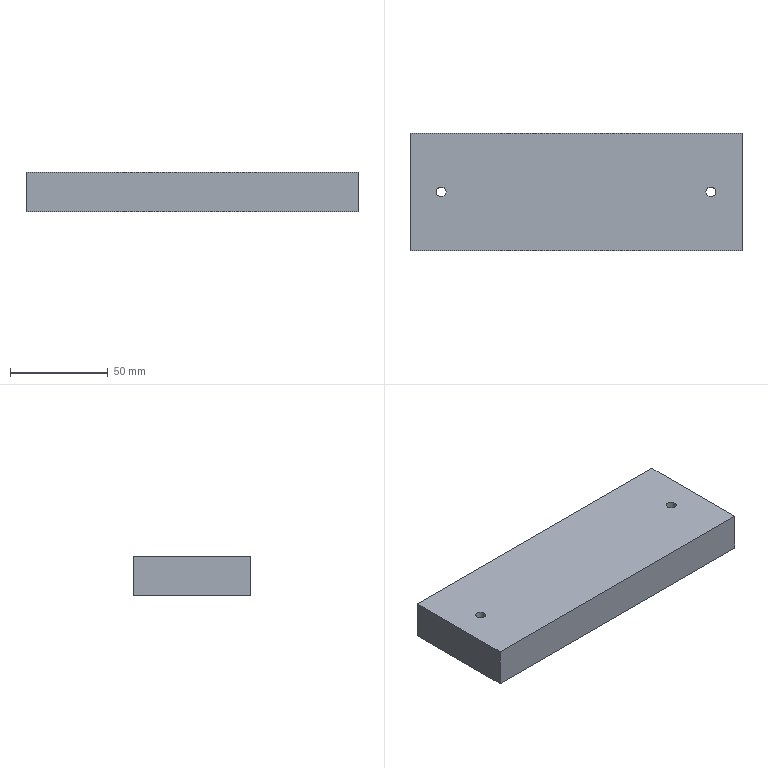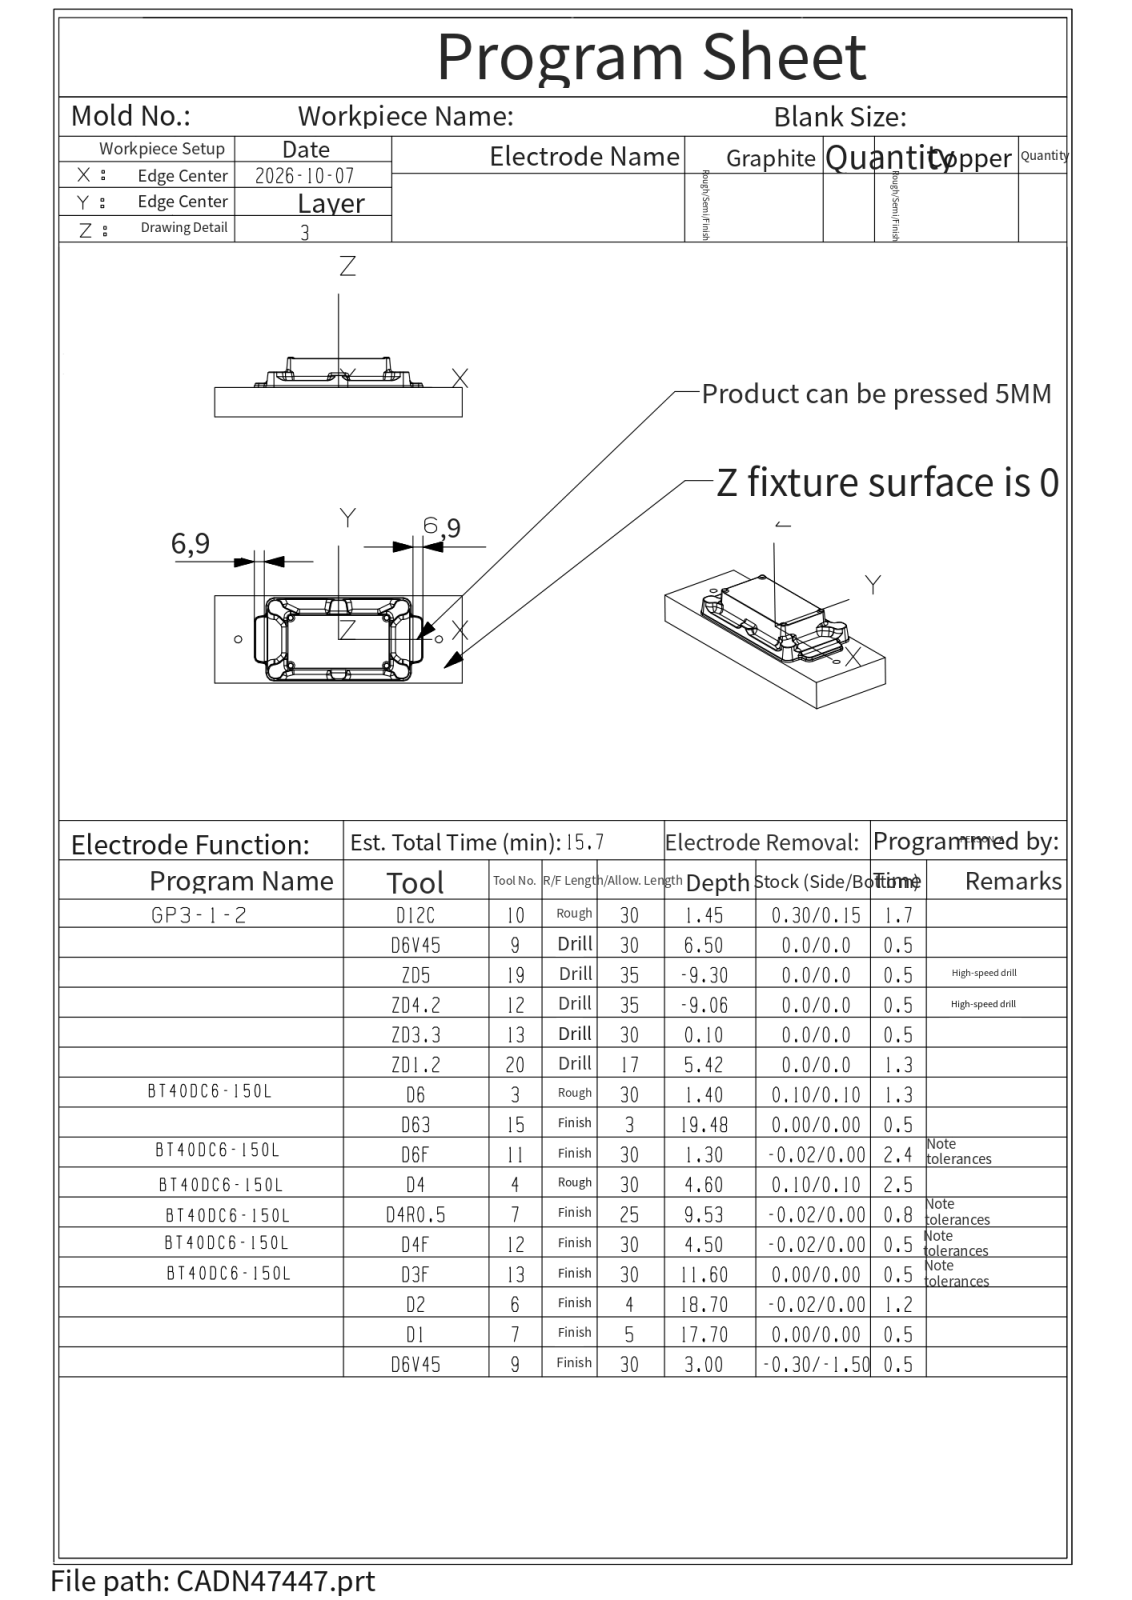NC program | NX | posted by the shop | part box 170 x 60 x 20 mm
Lines 9728 to 10588 of 17682:
T20 M06
T12
( name=R1    T=20 )
( XY = 0.00 )
( Z = 0.00 )
G00 G90 G54 X-52.788 Y-14.057 S10000 M03
G43 Z27.98 H20 M08
Z17.532
G01 X-52.766 Y-14.03 F1600.
G03 X-52.821 Y-13.467 I-.309 J.254
X-53.979 Y-13.468 I-.579 J-.706 F2000.
X-54.034 Y-14.031 I.254 J-.309
G01 X-54.01 Y-14.061
X-54.222 Y-14.52 Z17.504 F6000.
G02 X-54.36 Y-13.98 I.21 J.341 F1600.
X-53.334 Y-13.353 I1.084 J-.622 F2000.
X-52.44 Y-13.98 I-.271 J-1.337
X-52.574 Y-14.53 I-.341 J-.208
G01 X-52.418 Y-15.082 Z17.471 F6000.
X-52.409 Y-15.078 F1600.
G03 X-52.196 Y-14.554 I-.155 J.369
X-52.929 Y-13.606 I-2.151 J-.904 F2000.
X-53.874 Y-13.607 I-.471 J-.616
X-54.604 Y-14.554 I1.432 J-1.86
X-54.386 Y-15.08 I.369 J-.156
G01 X-54.493 Y-15.696 Z17.432 F6000.
G02 X-54.777 Y-15.208 I.103 J.386 F1600.
X-53.875 Y-13.716 I2.972 J-.777 F2000.
X-52.928 Y-13.714 I.474 J-.52
X-52.023 Y-15.209 I-2.052 J-2.264
X-52.308 Y-15.696 I-.387 J-.101
G01 X-52.251 Y-16.369 Z17.388 F6000.
X-52.248 Y-16.368 F1600.
G03 X-51.92 Y-15.907 I-.067 J.394
X-52.555 Y-14.256 I-4.413 J-.748 F2000.
X-53.126 Y-13.682 I-1.49 J-.913
X-53.752 Y-13.724 I-.284 J-.46
G01 X-53.895 Y-13.841
G03 X-54.611 Y-14.962 I2.227 J-2.212
G01 X-54.632 Y-15.018
G03 X-54.88 Y-15.908 I4.737 J-1.796
X-54.551 Y-16.374 I.394 J-.072
G01 X-54.542 Y-17.066 Z17.338 F6000.
X-54.547 F1600.
G02 X-54.917 Y-16.638 I.029 J.399
X-54.241 Y-14.397 I5.309 J-.379 F2000.
X-53.774 Y-13.832 I1.969 J-1.151
X-53.027 Y-13.831 I.374 J-.416
X-52.559 Y-14.397 I-1.49 J-1.707
X-51.883 Y-16.639 I-4.611 J-2.614
X-52.259 Y-17.066 I-.399 J-.028
G01 X-52.306 Y-17.731 Z17.288 F6000.
G03 X-51.906 Y-17.334 I0.0 J.4 F1600.
X-52.417 Y-14.821 I-6.2 J.048 F2000.
X-52.971 Y-13.967 I-2.853 J-1.244
X-53.814 Y-13.952 I-.428 J-.391
X-54.28 Y-14.612 I1.818 J-1.778
X-54.894 Y-17.348 I5.415 J-2.651
X-54.494 Y-17.742 I.4 J.006
G00 Z27.98
X-56.8 Y-22.456
Z17.238
G02 X-56.4 Y-22.056 I.4 J0.0 F1600.
G03 X-54.844 Y-20.5 I0.0 J1.556 F2000.
G01 Y-17.349
G02 X-54.17 Y-14.538 I6.236 J-.007
X-53.754 Y-13.991 I1.573 J-.764
X-53.054 Y-13.985 I.354 J-.423
X-52.629 Y-14.538 I-1.096 J-1.281
X-51.956 Y-17.352 I-5.614 J-2.829
G01 Y-23.287
G02 X-52.356 Y-23.687 I-.4 J0.0
G01 X-52.407 Z17.187 F6000.
G03 X-52.007 Y-23.287 I0.0 J.4 F1600.
G01 Y-17.356 F2000.
G03 X-52.638 Y-14.625 I-6.724 J-.114
X-53.029 Y-14.093 I-1.521 J-.71
X-53.775 Y-14.096 I-.371 J-.408
X-54.161 Y-14.623 I1.154 J-1.251
X-54.793 Y-17.36 I6.033 J-2.835
G01 Y-20.5
G02 X-56.4 Y-22.107 I-1.607 J0.0
G03 X-56.8 Y-22.507 I0.0 J-.4
G01 Y-22.557 Z17.137 F6000.
G02 X-56.4 Y-22.157 I.4 J0.0 F1600.
G03 X-54.743 Y-20.5 I0.0 J1.657 F2000.
G01 Y-17.36
G02 X-54.599 Y-16.125 I7.524 J-.254
G01 X-54.571 Y-15.986
G02 X-54.117 Y-14.635 I5.618 J-1.133
X-53.754 Y-14.166 I1.284 J-.617
X-53.054 Y-14.16 I.354 J-.423
X-52.773 Y-14.477 I-.692 J-.894
X-52.481 Y-15.104 I-3.173 J-1.86
X-52.057 Y-17.361 I-7.062 J-2.495
G01 Y-23.296
G02 X-52.457 Y-23.696 I-.4 J0.0
G01 X-52.507 Y-23.705 Z17.087 F6000.
G03 X-52.107 Y-23.305 I0.0 J.4 F1600.
G01 Y-17.365 F2000.
G03 X-52.429 Y-15.386 I-7.847 J-.262
X-52.73 Y-14.641 I-3.903 J-1.142
X-53.055 Y-14.246 I-1.112 J-.582
X-53.761 Y-14.258 I-.346 J-.429
X-54.135 Y-14.765 I.938 J-1.085
X-54.547 Y-16.093 I5.398 J-2.399
G01 X-54.566 Y-16.194
G03 X-54.693 Y-17.567 I7.355 J-1.373
G01 Y-20.503
G02 X-56.4 Y-22.207 I-1.707 J.003
G03 X-56.8 Y-22.607 I0.0 J-.4
G01 Y-22.654 Z17.036 F6000.
G02 X-56.4 Y-22.254 I.4 J0.0 F1600.
G03 X-54.646 Y-20.501 I0.0 J1.754 F2000.
G01 X-54.649 Y-20.485
Y-17.506
Y-17.478
G02 X-54.596 Y-16.697 I6.881 J-.079
X-54.175 Y-14.945 I6.526 J-.64
X-53.754 Y-14.34 I1.368 J-.502
X-53.054 Y-14.335 I.354 J-.422
X-52.682 Y-14.821 I-.802 J-.999
X-52.427 Y-15.528 I-3.972 J-1.83
X-52.154 Y-17.365 I-7.541 J-2.058
G01 Y-23.305
G02 X-52.554 Y-23.705 I-.4 J0.0
G01 X-52.595 Z16.986 F6000.
G03 X-52.195 Y-23.305 I0.0 J.4 F1600.
G01 Y-17.365 F2000.
G03 X-52.546 Y-15.245 I-7.534 J-.158
X-52.913 Y-14.55 I-1.966 J-.594
X-53.334 Y-14.301 I-.562 J-.469
X-53.854 Y-14.514 I-.047 J-.628
X-54.208 Y-15.118 I1.392 J-1.221
G01 X-54.252 Y-15.245
G03 X-54.606 Y-17.506 I7.093 J-2.267
G01 Y-20.496
X-54.605 Y-20.504
G02 X-56.4 Y-22.295 I-1.795 J.004
G03 X-56.8 Y-22.695 I0.0 J-.4
G01 Y-22.731 Z16.936 F6000.
G02 X-56.4 Y-22.331 I.4 J0.0 F1600.
G03 X-54.569 Y-20.505 I0.0 J1.831 F2000.
G01 X-54.571 Y-20.499
Y-17.365
G02 X-54.462 Y-16.234 I8.2 J-.219
G01 X-54.455 Y-16.199
X-54.452 Y-16.179
G02 X-54.173 Y-15.116 I5.314 J-.826
X-53.783 Y-14.538 I1.396 J-.524
X-53.054 Y-14.509 I.381 J-.401
X-52.773 Y-14.826 I-.684 J-.887
X-52.533 Y-15.386 I-1.967 J-1.174
G01 X-52.492 Y-15.528
G02 X-52.231 Y-17.365 I-7.283 J-1.97
G01 Y-23.305
G02 X-52.631 Y-23.705 I-.4 J0.0
G01 X-52.663 Z16.885 F6000.
G03 X-52.263 Y-23.305 I0.0 J.4 F1600.
G01 Y-17.365 F2000.
G03 X-52.48 Y-15.669 I-7.704 J-.125
X-52.746 Y-14.962 I-2.791 J-.646
X-53.054 Y-14.597 I-.982 J-.514
X-53.754 Y-14.602 I-.347 J-.427
X-54.175 Y-15.208 I.977 J-1.127
X-54.402 Y-16.038 I4.792 J-1.757
X-54.539 Y-17.53 I8.082 J-1.492
G01 Y-20.499
X-54.537 Y-20.505
G02 X-56.4 Y-22.363 I-1.863 J.005
G03 X-56.8 Y-22.763 I0.0 J-.4
G01 Y-22.79 Z16.835 F6000.
G02 X-56.4 Y-22.39 I.4 J0.0 F1600.
G03 X-54.51 Y-20.505 I0.0 J1.89 F2000.
G01 Y-20.499
Y-17.484
G02 X-54.34 Y-15.849 I7.911 J0.0
X-54.152 Y-15.245 I3.338 J-.705
X-53.754 Y-14.689 I1.302 J-.512
X-53.054 Y-14.684 I.354 J-.421
X-52.715 Y-15.104 I-.734 J-.937
G01 X-52.699 Y-15.139
G02 X-52.454 Y-15.882 I-2.788 J-1.329
G01 X-52.441 Y-15.952
G02 X-52.29 Y-17.365 I-7.648 J-1.528
G01 Y-23.305
G02 X-52.69 Y-23.705 I-.4 J0.0
G01 X-52.714 Z16.785 F6000.
G03 X-52.314 Y-23.305 I0.0 J.4 F1600.
G01 Y-17.365 F2000.
G03 X-52.491 Y-15.81 I-7.749 J-.095
X-52.765 Y-15.104 I-2.463 J-.546
X-53.083 Y-14.75 I-.946 J-.53
X-53.75 Y-14.773 I-.318 J-.449
X-54.11 Y-15.239 I.832 J-1.014
X-54.354 Y-16.027 I2.88 J-1.326
G01 X-54.371 Y-16.122
G03 X-54.486 Y-17.473 I7.849 J-1.35
G01 Y-20.499
Y-20.505
G02 X-56.4 Y-22.414 I-1.914 J.005
G03 X-56.8 Y-22.814 I0.0 J-.4
G01 Y-22.835 Z16.734 F6000.
G02 X-56.4 Y-22.435 I.4 J0.0 F1600.
G03 X-54.465 Y-20.505 I0.0 J1.935 F2000.
G01 X-54.466 Y-20.499
Y-17.455
G02 X-54.333 Y-16.012 I7.874 J0.0
X-54.107 Y-15.32 I2.733 J-.509
X-53.758 Y-14.867 I1.245 J-.597
X-53.054 Y-14.859 I.357 J-.418
X-52.734 Y-15.245 I-.687 J-.893
X-52.48 Y-15.952 I-2.317 J-1.231
X-52.335 Y-17.365 I-7.306 J-1.466
G01 Y-23.305
G02 X-52.735 Y-23.705 I-.4 J0.0
G01 X-52.753 Z16.684 F6000.
G03 X-52.353 Y-23.305 I0.0 J.4 F1600.
G01 Y-17.358 F2000.
G03 X-52.47 Y-16.093 I-7.244 J-.033
X-52.704 Y-15.386 I-2.796 J-.534
X-53.054 Y-14.946 I-1.112 J-.524
X-53.754 Y-14.951 I-.347 J-.427
X-54.096 Y-15.386 I.828 J-1.001
X-54.347 Y-16.182 I2.579 J-1.253
X-54.448 Y-17.438 I7.784 J-1.257
G01 X-54.449 Y-20.498
X-54.447 Y-20.506
G02 X-56.4 Y-22.453 I-1.953 J.006
G03 X-56.8 Y-22.853 I0.0 J-.4
G01 Y-22.867 Z16.634 F6000.
G02 X-56.4 Y-22.467 I.4 J0.0 F1600.
G03 X-54.433 Y-20.506 I0.0 J1.967 F2000.
G01 X-54.434 Y-17.511
G02 X-54.364 Y-16.376 I7.884 J.085
X-54.122 Y-15.528 I3.007 J-.398
X-53.747 Y-15.032 I1.204 J-.522
X-53.086 Y-15.009 I.346 J-.424
X-52.763 Y-15.367 I-.627 J-.89
X-52.473 Y-16.171 I-2.288 J-1.281
X-52.367 Y-17.359 I-6.259 J-1.157
G01 Y-23.305
G02 X-52.767 Y-23.705 I-.4 J0.0
G01 X-52.779 Z16.584 F6000.
G03 X-52.379 Y-23.305 I0.0 J.4 F1600.
G01 Y-17.361 F2000.
G03 X-52.45 Y-16.376 I-6.446 J.03
X-52.723 Y-15.528 I-2.804 J-.433
X-53.054 Y-15.12 I-1.043 J-.51
X-53.754 Y-15.126 I-.347 J-.427
X-54.147 Y-15.669 I.895 J-1.06
X-54.382 Y-16.61 I2.95 J-1.236
X-54.421 Y-17.463 I9.196 J-.852
G01 Y-20.506
G02 X-56.4 Y-22.479 I-1.979 J.006
G03 X-56.8 Y-22.879 I0.0 J-.4
G01 Y-22.888 Z16.533 F6000.
G02 X-56.4 Y-22.488 I.4 J0.0 F1600.
G03 X-54.412 Y-20.507 I0.0 J1.988 F2000.
G01 X-54.413 Y-17.42
G02 X-54.39 Y-16.797 I8.549 J.003
X-54.175 Y-15.818 I3.491 J-.254
X-53.793 Y-15.245 I1.422 J-.534
X-53.054 Y-15.208 I.391 J-.394
X-52.694 Y-15.669 I-.771 J-.971
X-52.441 Y-16.517 I-2.699 J-1.266
X-52.388 Y-17.349 I-6.013 J-.802
G01 Y-23.302
G02 X-52.788 Y-23.702 I-.4 J0.0
G01 X-52.795 Z16.483 F6000.
G03 X-52.395 Y-23.302 I0.0 J.4 F1600.
G01 Y-17.354 F2000.
G03 X-52.455 Y-16.517 I-5.006 J.059
X-52.742 Y-15.669 I-2.69 J-.436
X-53.061 Y-15.289 I-.987 J-.506
X-53.816 Y-15.349 I-.344 J-.456
X-54.218 Y-16.021 I1.259 J-1.209
X-54.404 Y-17.168 I3.639 J-1.178
X-54.407 Y-17.869 I87.413 J-.701
G01 Y-20.174
X-54.408 Y-20.191
Y-20.474
X-54.405 Y-20.507
G02 X-56.4 Y-22.495 I-1.995 J.007
G03 X-56.8 Y-22.895 I0.0 J-.4
G01 Y-22.899 Z16.433 F6000.
G02 X-56.4 Y-22.499 I.4 J0.0 F1600.
G03 X-54.401 Y-20.507 I0.0 J1.999 F2000.
G01 X-54.402 Y-19.82
X-54.403 Y-17.365
X-54.399 Y-17.153
G02 X-54.173 Y-15.986 I3.53 J-.078
X-53.754 Y-15.387 I1.385 J-.522
X-53.054 Y-15.382 I.354 J-.422
X-52.711 Y-15.81 I-.751 J-.952
X-52.462 Y-16.577 I-2.748 J-1.317
X-52.399 Y-17.274 I-3.798 J-.697
G01 Y-23.303
G02 X-52.799 Y-23.703 I-.4 J0.0
G01 X-52.8 Z16.382 F6000.
G03 X-52.4 Y-23.303 I0.0 J.4 F1600.
G01 Y-17.355 F2000.
G03 X-52.493 Y-16.508 I-3.954 J-.005
X-52.761 Y-15.81 I-2.626 J-.607
X-53.085 Y-15.446 I-.949 J-.518
X-53.762 Y-15.481 I-.317 J-.447
X-54.175 Y-16.08 I.977 J-1.116
X-54.401 Y-17.365 I3.385 J-1.256
G01 X-54.4 Y-17.435
Y-20.5
G02 X-54.407 Y-20.671 I-2.001 J0.0
X-56.39 Y-22.5 I-1.993 J.171
G03 X-56.788 Y-22.9 I.002 J-.4
G01 X-56.8 Z16.332 F6000.
G02 X-56.4 Y-22.5 I.4 J0.0 F1600.
G03 X-54.4 Y-20.5 I0.0 J2. F2000.
G01 Y-17.43
G02 X-54.175 Y-16.167 I3.547 J.02
X-53.754 Y-15.562 I1.395 J-.521
X-53.054 Y-15.556 I.354 J-.422
X-52.73 Y-15.952 I-.707 J-.909
X-52.493 Y-16.596 I-2.408 J-1.252
X-52.4 Y-17.43 I-3.877 J-.854
G01 Y-23.308
G02 X-52.8 Y-23.708 I-.4 J0.0
G01 Y-23.715 Z16.282 F6000.
G03 X-52.4 Y-23.315 I0.0 J.4 F1600.
G01 Y-17.48 F2000.
G03 X-52.469 Y-16.8 I-4.089 J-.069
X-52.7 Y-16.093 I-2.94 J-.571
X-53.054 Y-15.643 I-1.144 J-.535
X-53.779 Y-15.669 I-.348 J-.429
X-54.172 Y-16.247 I1.012 J-1.113
X-54.39 Y-17.284 I3.175 J-1.208
G01 X-54.4 Y-17.48
Y-20.5
G02 X-56.4 Y-22.5 I-2. J0.0
G03 X-56.8 Y-22.9 I0.0 J-.4
G01 Z16.231 F6000.
G02 X-56.4 Y-22.5 I.4 J0.0 F1600.
G01 X-56.395 F2000.
G03 X-54.4 Y-20.5 I-.005 J2.
G01 Y-17.509
G02 X-54.175 Y-16.341 I3.639 J-.095
X-53.754 Y-15.736 I1.408 J-.531
X-53.054 Y-15.73 I.354 J-.422
X-52.749 Y-16.093 I-.674 J-.875
X-52.493 Y-16.773 I-2.389 J-1.288
X-52.4 Y-17.568 I-3.829 J-.85
G01 Y-23.315
G02 X-52.8 Y-23.715 I-.4 J0.0
G01 Y-23.725 Z16.181 F6000.
G03 X-52.4 Y-23.325 I0.0 J.4 F1600.
G01 Y-17.647 F2000.
G03 X-52.45 Y-17.082 I-4.252 J-.09
X-52.718 Y-16.234 I-2.876 J-.443
X-53.054 Y-15.817 I-1.09 J-.534
X-53.754 Y-15.823 I-.347 J-.428
X-54.141 Y-16.351 I.909 J-1.071
X-54.385 Y-17.379 I2.976 J-1.249
G01 X-54.398 Y-17.572
X-54.4 Y-17.581
Y-20.5
G02 X-56.4 Y-22.5 I-2. J0.0
G03 X-56.8 Y-22.9 I0.0 J-.4
G01 Z16.131 F6000.
G02 X-56.4 Y-22.5 I.4 J0.0 F1600.
G01 X-56.395 F2000.
G03 X-54.4 Y-20.5 I-.005 J2.
G01 Y-17.736
X-54.392 Y-17.568
G02 X-54.177 Y-16.521 I3.426 J-.158
X-53.804 Y-15.952 I1.457 J-.547
X-53.054 Y-15.904 I.401 J-.39
X-52.69 Y-16.376 I-.813 J-1.002
X-52.465 Y-17.082 I-2.778 J-1.277
X-52.4 Y-17.738 I-4.22 J-.747
G01 Y-23.334
G02 X-52.8 Y-23.734 I-.4 J0.0
G01 Z16.08 F6000.
G03 X-52.4 Y-23.334 I0.0 J.4 F1600.
G01 Y-17.824 F2000.
G03 X-52.493 Y-17.037 I-3.859 J-.057
X-52.737 Y-16.376 I-2.571 J-.573
X-53.054 Y-15.991 I-1.027 J-.524
X-53.754 Y-15.998 I-.347 J-.428
X-54.175 Y-16.603 I.989 J-1.136
X-54.382 Y-17.509 I3.189 J-1.204
G01 X-54.391 Y-17.647
X-54.4 Y-17.785
Y-20.5
G02 X-56.4 Y-22.5 I-2. J0.0
G03 X-56.8 Y-22.9 I0.0 J-.4
G01 Z16.03 F6000.
G02 X-56.4 Y-22.5 I.4 J0.0 F1600.
G01 X-56.395 F2000.
G03 X-54.4 Y-20.5 I-.005 J2.
G01 Y-17.842
X-54.398 Y-17.833
X-54.393 Y-17.727
G02 X-54.161 Y-16.658 I3.41 J-.181
X-53.764 Y-16.093 I1.346 J-.522
X-53.054 Y-16.078 I.364 J-.414
X-52.698 Y-16.533 I-.817 J-1.006
X-52.447 Y-17.361 I-2.704 J-1.271
X-52.4 Y-17.912 I-4.297 J-.644
G01 Y-23.344
G02 X-52.8 Y-23.744 I-.4 J0.0
G01 Z15.98 F6000.
G03 X-52.4 Y-23.344 I0.0 J.4 F1600.
G01 Y-18.001 F2000.
G03 X-52.633 Y-16.767 I-3.514 J-.025
X-53.054 Y-16.165 I-1.346 J-.493
X-53.754 Y-16.172 I-.346 J-.428
X-54.175 Y-16.777 I.983 J-1.132
X-54.387 Y-17.727 I3.3 J-1.234
G01 X-54.4 Y-17.996
Y-20.5
G02 X-56.4 Y-22.5 I-2. J0.0
G03 X-56.8 Y-22.9 I0.0 J-.4
G01 Z15.929 F6000.
G02 X-56.4 Y-22.5 I.4 J0.0 F1600.
G01 X-56.395 F2000.
G03 X-54.4 Y-20.5 I-.005 J2.
G01 Y-18.071
X-54.386 Y-17.829
G02 X-54.145 Y-16.8 I3.149 J-.192
X-53.754 Y-16.259 I1.294 J-.525
X-53.054 Y-16.252 I.355 J-.422
X-52.729 Y-16.65 I-.767 J-.957
X-52.456 Y-17.481 I-2.504 J-1.283
X-52.4 Y-18.142 I-4.25 J-.693
G01 Y-23.354
G02 X-52.8 Y-23.754 I-.4 J0.0
G01 Y-23.763 Z15.879 F6000.
G03 X-52.4 Y-23.363 I0.0 J.4 F1600.
G01 Y-18.214 F2000.
G03 X-52.47 Y-17.482 I-4.394 J-.052
X-52.695 Y-16.8 I-3.297 J-.709
X-53.054 Y-16.339 I-1.21 J-.572
X-53.781 Y-16.367 I-.348 J-.434
X-54.194 Y-17.009 I1.066 J-1.141
G01 X-54.219 Y-17.082
G03 X-54.386 Y-17.93 I3.031 J-1.038
X-54.4 Y-18.168 I2.695 J-.272
G01 Y-20.5
G02 X-56.4 Y-22.5 I-2. J0.0
G03 X-56.8 Y-22.9 I0.0 J-.4
G01 Z15.829 F6000.
G02 X-56.4 Y-22.5 I.4 J0.0 F1600.
G01 X-56.395 F2000.
G03 X-54.4 Y-20.5 I-.005 J2.
G01 Y-18.213
X-54.388 Y-18.001
G02 X-54.175 Y-17.038 I3.534 J-.276
X-53.824 Y-16.492 I1.519 J-.589
X-53.334 Y-16.306 I.444 J-.431
X-52.904 Y-16.569 I-.138 J-.709
X-52.575 Y-17.184 I-1.568 J-1.234
X-52.4 Y-18.302 I-3.374 J-1.101
G01 Y-23.363
G02 X-52.8 Y-23.763 I-.4 J0.0
G01 Y-23.773 Z15.778 F6000.
G03 X-52.4 Y-23.373 I0.0 J.4 F1600.
G01 Y-18.389 F2000.
G03 X-52.459 Y-17.73 I-4.154 J-.038
X-52.712 Y-16.941 I-3.01 J-.531
X-53.054 Y-16.514 I-1.185 J-.597
X-53.754 Y-16.521 I-.346 J-.429
X-54.155 Y-17.082 I.931 J-1.088
X-54.394 Y-18.213 I3.087 J-1.243
G01 X-54.4 Y-18.347
Y-20.5
G02 X-56.4 Y-22.5 I-2. J0.0
G03 X-56.8 Y-22.9 I0.0 J-.4
G01 Z15.728 F6000.
G02 X-56.4 Y-22.5 I.4 J0.0 F1600.
G01 X-56.395 F2000.
G03 X-54.4 Y-20.5 I-.005 J2.
G01 Y-18.433
X-54.389 Y-18.21
G02 X-54.226 Y-17.365 I3.289 J-.197
G01 X-54.201 Y-17.29
G02 X-53.805 Y-16.647 I1.586 J-.533
X-53.054 Y-16.601 I.402 J-.397
X-52.686 Y-17.082 I-.877 J-1.05
X-52.463 Y-17.789 I-2.933 J-1.314
X-52.4 Y-18.495 I-4.116 J-.724
G01 Y-23.373
G02 X-52.8 Y-23.773 I-.4 J0.0
G01 Z15.678 F6000.
G03 X-52.4 Y-23.373 I0.0 J.4 F1600.
G01 Y-18.566 F2000.
G03 X-52.459 Y-17.906 I-4.105 J-.032
X-52.732 Y-17.082 I-2.777 J-.464
X-53.054 Y-16.688 I-1.102 J-.57
X-53.754 Y-16.695 I-.346 J-.428
X-54.175 Y-17.3 I.982 J-1.131
X-54.392 Y-18.354 I3.187 J-1.204
G01 X-54.4 Y-18.492
Y-20.5
G02 X-56.4 Y-22.5 I-2. J0.0
G03 X-56.8 Y-22.9 I0.0 J-.4
G01 Z15.627 F6000.
G02 X-56.4 Y-22.5 I.4 J0.0 F1600.
G01 X-56.395 F2000.
G03 X-54.4 Y-20.5 I-.005 J2.
G01 Y-18.601
X-54.393 Y-18.425
G02 X-54.165 Y-17.365 I3.448 J-.187
X-53.776 Y-16.8 I1.386 J-.537
X-53.054 Y-16.775 I.375 J-.405
X-52.633 Y-17.378 I-.937 J-1.102
X-52.468 Y-17.93 I-3.778 J-1.427
X-52.4 Y-18.65 I-4.466 J-.787
G01 Y-23.382
G02 X-52.8 Y-23.782 I-.4 J0.0
G01 Y-23.79 Z15.577 F6000.
G03 X-52.4 Y-23.39 I0.0 J.4 F1600.
G01 Y-18.737 F2000.
G03 X-52.429 Y-18.284 I-4.932 J-.089
X-52.677 Y-17.365 I-3.094 J-.341
X-53.054 Y-16.863 I-1.27 J-.56
X-53.754 Y-16.869 I-.347 J-.426
X-54.175 Y-17.474 I.987 J-1.134
X-54.392 Y-18.495 I3.322 J-1.238
G01 X-54.397 Y-18.593
X-54.4 Y-18.637
Y-20.5
G02 X-56.4 Y-22.5 I-2. J0.0
G03 X-56.8 Y-22.9 I0.0 J-.4
G01 Z15.527 F6000.
G02 X-56.4 Y-22.5 I.4 J0.0 F1600.
G01 X-56.395 F2000.
G03 X-54.4 Y-20.5 I-.005 J2.
G01 Y-18.778
X-54.393 Y-18.637
G02 X-54.15 Y-17.506 I3.295 J-.118
X-53.754 Y-16.956 I1.325 J-.535
X-53.054 Y-16.95 I.354 J-.42
X-52.708 Y-17.388 I-.838 J-1.016
X-52.454 Y-18.195 I-2.554 J-1.248
X-52.4 Y-18.825 I-4.45 J-.698
G01 Y-23.39
G02 X-52.8 Y-23.79 I-.4 J0.0
G01 Z15.476 F6000.
G03 X-52.4 Y-23.39 I0.0 J.4 F1600.
G01 Y-18.912 F2000.
G03 X-52.465 Y-18.213 I-4.443 J-.061
X-52.691 Y-17.506 I-3.216 J-.64
X-53.054 Y-17.037 I-1.262 J-.6
X-53.79 Y-17.071 I-.349 J-.435
X-54.198 Y-17.717 I1.12 J-1.159
G01 X-54.222 Y-17.789
G03 X-54.387 Y-18.637 I3.011 J-1.026
X-54.4 Y-18.866 I2.623 J-.262
G01 Y-20.5
G02 X-56.4 Y-22.5 I-2. J0.0
G03 X-56.8 Y-22.9 I0.0 J-.4
G01 Z15.426 F6000.
G02 X-56.4 Y-22.5 I.4 J0.0 F1600.
G01 X-56.395 F2000.
G03 X-54.4 Y-20.5 I-.005 J2.
G01 Y-18.915
X-54.391 Y-18.76
G02 X-54.175 Y-17.737 I3.474 J-.198
X-53.754 Y-17.13 I1.407 J-.527
X-53.054 Y-17.125 I.354 J-.419
X-52.74 Y-17.506 I-.814 J-.988
X-52.484 Y-18.213 I-2.318 J-1.24
X-52.4 Y-18.999 I-4.02 J-.826
G01 Y-23.4
G02 X-52.8 Y-23.8 I-.4 J0.0
G01 Z15.376 F6000.
G03 X-52.4 Y-23.4 I0.0 J.4 F1600.
G01 Y-19.086 F2000.
G03 X-52.47 Y-18.354 I-4.639 J-.077
X-52.633 Y-17.813 I-4.156 J-.953
X-53.054 Y-17.212 I-1.386 J-.523
X-53.762 Y-17.224 I-.347 J-.425
X-54.159 Y-17.789 I.967 J-1.103
X-54.385 Y-18.778 I3.018 J-1.208
G01 X-54.4 Y-18.977
Y-20.5
G02 X-56.4 Y-22.5 I-2. J0.0
G03 X-56.8 Y-22.9 I0.0 J-.4
G01 Z15.325 F6000.
G02 X-56.4 Y-22.5 I.4 J0.0 F1600.
G01 X-56.395 F2000.
G03 X-54.4 Y-20.5 I-.005 J2.
G01 Y-19.122
X-54.39 Y-18.919
G02 X-54.175 Y-17.91 I3.437 J-.203
X-53.754 Y-17.305 I1.398 J-.522
X-53.054 Y-17.3 I.353 J-.419
X-52.682 Y-17.789 I-.917 J-1.082
X-52.451 Y-18.567 I-2.774 J-1.246
X-52.4 Y-19.173 I-4.134 J-.655
G01 Y-23.409
G02 X-52.8 Y-23.809 I-.4 J0.0
G01 Z15.275 F6000.
G03 X-52.4 Y-23.409 I0.0 J.4 F1600.
G01 Y-19.261 F2000.
G03 X-52.444 Y-18.697 I-4.528 J-.071
X-52.668 Y-17.907 I-3.01 J-.426
X-53.054 Y-17.387 I-1.32 J-.576
X-53.754 Y-17.392 I-.348 J-.424
X-54.144 Y-17.93 I.926 J-1.081
X-54.386 Y-18.968 I2.892 J-1.22
G01 X-54.4 Y-19.198
Y-20.5
G02 X-56.4 Y-22.5 I-2. J0.0
G03 X-56.8 Y-22.9 I0.0 J-.4
G01 Z15.225 F6000.
G02 X-56.4 Y-22.5 I.4 J0.0 F1600.
G01 X-56.395 F2000.
G03 X-54.4 Y-20.5 I-.005 J2.
G01 Y-19.299
G02 X-54.387 Y-19.061 I3.099 J-.054
G01 X-54.373 Y-18.912
G02 X-54.218 Y-18.213 I2.955 J-.285
G01 X-54.194 Y-18.14
G02 X-53.779 Y-17.498 I1.477 J-.499
X-53.054 Y-17.475 I.376 J-.404
X-52.633 Y-18.073 I-.972 J-1.13
X-52.467 Y-18.637 I-3.734 J-1.406
X-52.4 Y-19.317 I-4.534 J-.791
G01 Y-23.418
G02 X-52.8 Y-23.818 I-.4 J0.0
G01 Z15.174 F6000.
G03 X-52.4 Y-23.418 I0.0 J.4 F1600.
G01 Y-19.435 F2000.
G03 X-52.459 Y-18.778 I-4.3 J-.056
X-52.673 Y-18.071 I-2.83 J-.471
X-53.054 Y-17.562 I-1.292 J-.569
X-53.754 Y-17.566 I-.348 J-.423
X-54.175 Y-18.172 I.985 J-1.133
X-54.386 Y-19.114 I3.239 J-1.22
G01 X-54.4 Y-19.407
Y-20.5
G02 X-56.4 Y-22.5 I-2. J0.0
G03 X-56.8 Y-22.9 I0.0 J-.4
G01 Z15.124 F6000.
G02 X-56.4 Y-22.5 I.4 J0.0 F1600.
G01 X-56.395 F2000.
G03 X-54.4 Y-20.5 I-.005 J2.
G01 Y-19.476
G02 X-54.384 Y-19.202 I3.414 J-.062
X-54.154 Y-18.213 I3.147 J-.21
X-53.754 Y-17.653 I1.351 J-.541
X-53.054 Y-17.65 I.352 J-.42
X-52.655 Y-18.198 I-.946 J-1.108
X-52.44 Y-18.992 I-2.934 J-1.221
X-52.4 Y-19.522 I-4.365 J-.592
G01 Y-23.418
G02 X-52.8 Y-23.818 I-.4 J0.0
G01 Y-23.824 Z15.074 F6000.
G03 X-52.4 Y-23.424 I0.0 J.4 F1600.
G01 Y-19.609 F2000.
G03 X-52.633 Y-18.334 I-3.576 J.006
X-53.054 Y-17.737 I-1.397 J-.539
X-53.754 Y-17.74 I-.349 J-.423
X-54.114 Y-18.213 I.881 J-1.044
X-54.365 Y-19.115 I2.679 J-1.231
X-54.4 Y-19.591 I3.532 J-.497
G01 Y-20.5
G02 X-56.4 Y-22.5 I-2. J0.0
G03 X-56.8 Y-22.9 I0.0 J-.4
G01 Z15.023 F6000.
G02 X-56.4 Y-22.5 I.4 J0.0 F1600.
G01 X-56.395 F2000.
G03 X-54.4 Y-20.5 I-.005 J2.
G01 Y-19.622
X-54.389 Y-19.414
G02 X-54.175 Y-18.433 I3.438 J-.235
X-53.754 Y-17.827 I1.419 J-.536
X-53.054 Y-17.825 I.352 J-.42
X-52.633 Y-18.42 I-.983 J-1.14
X-52.4 Y-19.696 I-3.361 J-1.273
G01 Y-23.427
G02 X-52.8 Y-23.827 I-.4 J0.0
G01 Y-23.83 Z14.973 F6000.
G03 X-52.4 Y-23.43 I0.0 J.4 F1600.
G01 Y-19.75 F2000.
G03 X-52.633 Y-18.507 I-3.576 J-.028
X-53.054 Y-17.912 I-1.395 J-.54
X-53.773 Y-17.93 I-.35 J-.424
X-54.159 Y-18.485 I1.002 J-1.11
X-54.374 Y-19.349 I3.021 J-1.208
G01 X-54.386 Y-19.468
X-54.4 Y-19.741
Y-20.5
G02 X-56.4 Y-22.5 I-2. J0.0
G03 X-56.8 Y-22.9 I0.0 J-.4
G01 Z14.923 F6000.
G02 X-56.4 Y-22.5 I.4 J0.0 F1600.
G01 X-56.395 F2000.
G03 X-54.4 Y-20.5 I-.005 J2.
G01 Y-19.829
G02 X-54.378 Y-19.477 I3.741 J-.06
G01 X-54.362 Y-19.348
G02 X-54.117 Y-18.48 I2.966 J-.368
X-53.754 Y-18.002 I1.24 J-.563
X-53.054 Y-18. I.351 J-.421
X-52.633 Y-18.594 I-.969 J-1.132
X-52.4 Y-19.838 I-3.343 J-1.27
G01 Y-23.433
G02 X-52.8 Y-23.833 I-.4 J0.0
G01 Y-23.837 Z14.872 F6000.
G03 X-52.4 Y-23.437 I0.0 J.4 F1600.
G01 Y-19.958 F2000.
G03 X-52.633 Y-18.68 I-3.6 J.003
X-53.054 Y-18.087 I-1.407 J-.552
X-53.754 Y-18.089 I-.35 J-.423
X-54.149 Y-18.637 I.939 J-1.091
X-54.382 Y-19.623 I2.857 J-1.198
X-54.4 Y-19.909 I3.588 J-.364
G01 Y-20.5
G02 X-56.4 Y-22.5 I-2. J0.0
G03 X-56.8 Y-22.9 I0.0 J-.4
G01 Z14.822 F6000.
G02 X-56.4 Y-22.5 I.4 J0.0 F1600.
G01 X-56.395 F2000.
G03 X-54.4 Y-20.5 I-.005 J2.
G01 Y-19.997
G02 X-54.374 Y-19.624 I3.534 J-.06
X-54.109 Y-18.637 I2.963 J-.266
X-53.754 Y-18.176 I1.245 J-.59
X-53.035 Y-18.191 I.351 J-.421
X-52.607 Y-18.835 I-1.06 J-1.167
X-52.4 Y-20.045 I-3.446 J-1.213
G01 Y-23.44
G02 X-52.8 Y-23.84 I-.4 J0.0
G01 Y-23.845 Z14.772 F6000.
G03 X-52.4 Y-23.445 I0.0 J.4 F1600.
G01 Y-20.103 F2000.
G03 X-52.633 Y-18.854 I-3.55 J-.016
X-53.054 Y-18.262 I-1.398 J-.548
X-53.754 Y-18.263 I-.35 J-.422
X-54.122 Y-18.752 I.901 J-1.06
X-54.362 Y-19.607 I2.707 J-1.219
G01 X-54.38 Y-19.76
G03 X-54.4 Y-20.132 I4.284 J-.412
G01 Y-20.5
G02 X-56.4 Y-22.5 I-2. J0.0
G03 X-56.8 Y-22.9 I0.0 J-.4
G01 Z14.721 F6000.
G02 X-56.4 Y-22.5 I.4 J0.0 F1600.
G01 X-56.395 F2000.
G03 X-54.4 Y-20.5 I-.005 J2.
G01 Y-20.174
G02 X-54.384 Y-19.88 I2.668 J0.0
G01 X-54.377 Y-19.821
X-54.373 Y-19.767
X-54.37 Y-19.761
G02 X-54.158 Y-18.919 I3.021 J-.313
X-53.759 Y-18.354 I1.363 J-.539
X-53.054 Y-18.35 I.355 J-.418
X-52.633 Y-18.941 I-.986 J-1.147
X-52.493 Y-19.392 I-3.953 J-1.475
X-52.4 Y-20.187 I-3.898 J-.858
G01 Y-23.445
G02 X-52.8 Y-23.845 I-.4 J0.0
G01 Z14.671 F6000.
G03 X-52.4 Y-23.445 I0.0 J.4 F1600.
G01 Y-20.307 F2000.
G03 X-52.493 Y-19.478 I-4.012 J-.03
X-52.685 Y-18.919 I-2.768 J-.638
X-53.054 Y-18.437 I-1.218 J-.549
X-53.823 Y-18.495 I-.354 J-.436
X-54.175 Y-19.043 I1.185 J-1.149
X-54.39 Y-20.05 I3.178 J-1.205
G01 X-54.398 Y-20.2
X-54.4 Y-20.209
Y-20.5
G02 X-56.4 Y-22.5 I-2. J0.0
G03 X-56.8 Y-22.9 I0.0 J-.4
G01 Z14.621 F6000.
G02 X-56.4 Y-22.5 I.4 J0.0 F1600.
G01 X-56.395 F2000.
G03 X-54.4 Y-20.5 I-.005 J2.
G01 Y-20.297
X-54.398 Y-20.288
X-54.385 Y-20.09
G02 X-54.17 Y-19.117 I3.262 J-.211
X-53.754 Y-18.525 I1.414 J-.55
X-53.054 Y-18.524 I.351 J-.422
X-52.659 Y-19.061 I-.918 J-1.089
X-52.442 Y-19.839 I-2.846 J-1.214
X-52.4 Y-20.394 I-4.935 J-.649
G01 Y-23.453
G02 X-52.8 Y-23.853 I-.4 J0.0
G01 Z14.57 F6000.
G03 X-52.4 Y-23.453 I0.0 J.4 F1600.
G01 Y-20.447 F2000.
G03 X-52.422 Y-20.095 I-5.659 J-.176
X-52.633 Y-19.201 I-3.312 J-.31
X-53.023 Y-18.637 I-1.433 J-.574
X-53.754 Y-18.612 I-.38 J-.401
X-54.175 Y-19.218 I.989 J-1.135
X-54.387 Y-20.175 I3.185 J-1.208
G01 X-54.386 Y-20.191
G03 X-54.4 Y-20.481 I4.735 J-.376
G01 Y-20.5
G02 X-56.4 Y-22.5 I-2. J0.0
G03 X-56.8 Y-22.9 I0.0 J-.4
G01 Z14.52 F6000.
G02 X-56.4 Y-22.5 I.4 J0.0 F1600.
G01 X-56.395 F2000.
G03 X-54.4 Y-20.528 I-.005 J2.
G01 X-54.399 Y-20.474
X-54.38 Y-20.191
X-54.374 Y-20.147
G02 X-54.175 Y-19.305 I3.159 J-.304
G01 X-54.128 Y-19.202
G02 X-53.77 Y-18.712 I1.258 J-.544
X-53.007 Y-18.734 I.37 J-.425
X-52.633 Y-19.288 I-1.142 J-1.173
X-52.4 Y-20.568 I-3.32 J-1.266
G01 Y-23.453
G02 X-52.8 Y-23.853 I-.4 J0.0
G01 Y-23.861 Z14.47 F6000.
G03 X-52.4 Y-23.461 I0.0 J.4 F1600.
G01 Y-20.655 F2000.
G03 X-52.633 Y-19.375 I-3.55 J.015
X-53.054 Y-18.786 I-1.404 J-.559
X-53.754 I-.351 J-.422
X-54.175 Y-19.392 I.998 J-1.142
X-54.397 Y-20.507 I3.268 J-1.229
G01 X-54.399 Y-20.572
G02 X-54.918 Y-21.843 I-1.966 J.061
X-56.4 Y-22.5 I-1.482 J1.343
G03 X-56.8 Y-22.9 I0.0 J-.4
G01 Z14.419 F6000.
G02 X-56.4 Y-22.5 I.4 J0.0 F1600.
G01 X-56.395 F2000.
G03 X-55.297 Y-22.168 I-.005 J2.
X-54.398 Y-20.616 I-1.068 J1.655
G01 X-54.395 Y-20.562
G02 X-54.36 Y-20.191 I4.673 J-.256
X-54.113 Y-19.343 I2.943 J-.397
X-53.754 Y-18.873 I1.237 J-.572
X-53.002 Y-18.914 I.354 J-.437
X-52.586 Y-19.59 I-1.227 J-1.222
X-52.4 Y-20.743 I-3.457 J-1.149
G01 Y-23.461
G02 X-52.8 Y-23.861 I-.4 J0.0
G01 Z14.369 F6000.
G03 X-52.4 Y-23.461 I0.0 J.4 F1600.
G01 Y-20.792 F2000.
G03 X-52.556 Y-19.767 I-3.701 J-.041
G01 X-52.605 Y-19.626
G03 X-52.998 Y-19.003 I-1.57 J-.553
X-53.783 Y-18.986 I-.402 J-.401
X-54.175 Y-19.566 I1.021 J-1.112
X-54.389 Y-20.545 I3.116 J-1.195
G01 X-54.391 Y-20.563
X-54.394 Y-20.615
X-54.399 Y-20.686
X-54.401 Y-20.715
X-54.404 Y-20.757